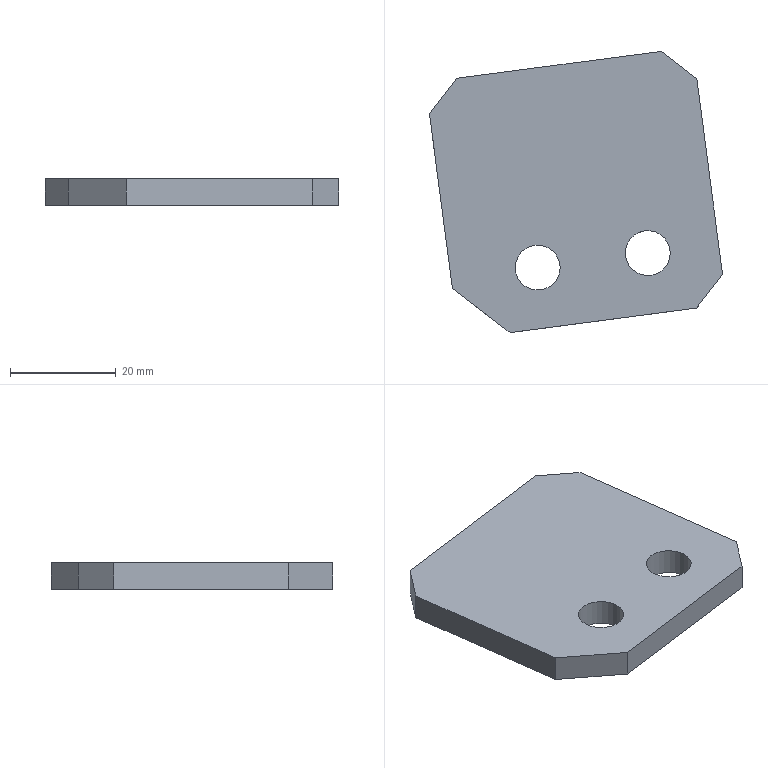Part | STEP file | gslz 2016.10.28-13_id538_x_t | 1 solid | 12 faces | box 55.431 x 53.187 x 5 mm | volume 11431 mm3 | plane 10 | cylinder 2 | commonest cylinder face diameters 8.5 x2
STEP:
#1=CARTESIAN_POINT('',(0.,0.,0.));
#2=DIRECTION('',(0.,0.,1.));
#3=DIRECTION('',(1.,0.,0.));
#4=AXIS2_PLACEMENT_3D('',#1,#2,#3);
#5=CARTESIAN_POINT('',(79.888,120.388,-99.));
#6=VERTEX_POINT('',#5);
#7=CARTESIAN_POINT('',(41.221,115.298,-99.));
#8=VERTEX_POINT('',#7);
#9=CARTESIAN_POINT('',(-1381.417,-71.996,-99.));
#10=DIRECTION('',(-0.9914,-0.1305,0.));
#11=VECTOR('',#10,1.);
#12=LINE('',#9,#11);
#13=CARTESIAN_POINT('',(-1381.417,-71.996,-99.));
#14=DIRECTION('',(-0.1305,0.9914,0.));
#15=DIRECTION('',(-0.9914,-0.1305,0.));
#16=AXIS2_PLACEMENT_3D('',#13,#14,#15);
#17=PLANE('',#16);
#18=CARTESIAN_POINT('',(0.,0.));
#19=DIRECTION('',(1.,0.));
#20=VECTOR('',#19,1.);
#21=LINE('',#18,#20);
#22=(GEOMETRIC_REPRESENTATION_CONTEXT(2)PARAMETRIC_REPRESENTATION_CONTEXT()REPRESENTATION_CONTEXT('',''));
#23=DEFINITIONAL_REPRESENTATION('',(#21),#22);
#24=PCURVE('',#17,#23);
#25=CARTESIAN_POINT('',(-1376.131,-112.149,-99.));
#26=DIRECTION('',(0.,0.,-1.));
#27=DIRECTION('',(-1.,0.,0.));
#28=AXIS2_PLACEMENT_3D('',#25,#26,#27);
#29=PLANE('',#28);
#30=CARTESIAN_POINT('',(5.286,40.154));
#31=DIRECTION('',(0.9914,-0.1305));
#32=VECTOR('',#31,1.);
#33=LINE('',#30,#32);
#34=(GEOMETRIC_REPRESENTATION_CONTEXT(2)PARAMETRIC_REPRESENTATION_CONTEXT()REPRESENTATION_CONTEXT('',''));
#35=DEFINITIONAL_REPRESENTATION('',(#33),#34);
#36=PCURVE('',#29,#35);
#37=SURFACE_CURVE('',#12,(#24,#36),.PCURVE_S1.);
#38=EDGE_CURVE('',#6,#8,#37,.T.);
#39=ORIENTED_EDGE('',*,*,#38,.T.);
#40=CARTESIAN_POINT('',(41.221,115.298,-94.));
#41=VERTEX_POINT('',#40);
#42=CARTESIAN_POINT('',(41.221,115.298,-94.));
#43=DIRECTION('',(0.,0.,1.));
#44=VECTOR('',#43,1.);
#45=LINE('',#42,#44);
#46=CARTESIAN_POINT('',(-1434.914,5.));
#47=DIRECTION('',(0.,1.));
#48=VECTOR('',#47,1.);
#49=LINE('',#46,#48);
#50=(GEOMETRIC_REPRESENTATION_CONTEXT(2)PARAMETRIC_REPRESENTATION_CONTEXT()REPRESENTATION_CONTEXT('',''));
#51=DEFINITIONAL_REPRESENTATION('',(#49),#50);
#52=PCURVE('',#17,#51);
#53=CARTESIAN_POINT('',(36.056,108.566,-267.));
#54=DIRECTION('',(0.7934,-0.6088,0.));
#55=DIRECTION('',(0.,0.,-1.));
#56=AXIS2_PLACEMENT_3D('',#53,#54,#55);
#57=PLANE('',#56);
#58=CARTESIAN_POINT('',(-173.,8.485));
#59=DIRECTION('',(-1.,0.));
#60=VECTOR('',#59,1.);
#61=LINE('',#58,#60);
#62=(GEOMETRIC_REPRESENTATION_CONTEXT(2)PARAMETRIC_REPRESENTATION_CONTEXT()REPRESENTATION_CONTEXT('',''));
#63=DEFINITIONAL_REPRESENTATION('',(#61),#62);
#64=PCURVE('',#57,#63);
#65=SURFACE_CURVE('',#45,(#52,#64),.PCURVE_S1.);
#66=EDGE_CURVE('',#8,#41,#65,.T.);
#67=ORIENTED_EDGE('',*,*,#66,.T.);
#68=CARTESIAN_POINT('',(79.888,120.388,-94.));
#69=VERTEX_POINT('',#68);
#70=CARTESIAN_POINT('',(-1381.417,-71.996,-94.));
#71=DIRECTION('',(-0.9914,-0.1305,0.));
#72=VECTOR('',#71,1.);
#73=LINE('',#70,#72);
#74=CARTESIAN_POINT('',(0.,5.));
#75=DIRECTION('',(1.,0.));
#76=VECTOR('',#75,1.);
#77=LINE('',#74,#76);
#78=(GEOMETRIC_REPRESENTATION_CONTEXT(2)PARAMETRIC_REPRESENTATION_CONTEXT()REPRESENTATION_CONTEXT('',''));
#79=DEFINITIONAL_REPRESENTATION('',(#77),#78);
#80=PCURVE('',#17,#79);
#81=CARTESIAN_POINT('',(-1376.131,-112.149,-94.));
#82=DIRECTION('',(0.,0.,-1.));
#83=DIRECTION('',(-1.,0.,0.));
#84=AXIS2_PLACEMENT_3D('',#81,#82,#83);
#85=PLANE('',#84);
#86=CARTESIAN_POINT('',(5.286,40.154));
#87=DIRECTION('',(0.9914,-0.1305));
#88=VECTOR('',#87,1.);
#89=LINE('',#86,#88);
#90=(GEOMETRIC_REPRESENTATION_CONTEXT(2)PARAMETRIC_REPRESENTATION_CONTEXT()REPRESENTATION_CONTEXT('',''));
#91=DEFINITIONAL_REPRESENTATION('',(#89),#90);
#92=PCURVE('',#85,#91);
#93=SURFACE_CURVE('',#73,(#80,#92),.PCURVE_S1.);
#94=EDGE_CURVE('',#69,#41,#93,.T.);
#95=ORIENTED_EDGE('',*,*,#94,.F.);
#96=CARTESIAN_POINT('',(79.888,120.388,-99.));
#97=DIRECTION('',(0.,0.,-1.));
#98=VECTOR('',#97,1.);
#99=LINE('',#96,#98);
#100=CARTESIAN_POINT('',(-1473.914,0.));
#101=DIRECTION('',(0.,-1.));
#102=VECTOR('',#101,1.);
#103=LINE('',#100,#102);
#104=(GEOMETRIC_REPRESENTATION_CONTEXT(2)PARAMETRIC_REPRESENTATION_CONTEXT()REPRESENTATION_CONTEXT('',''));
#105=DEFINITIONAL_REPRESENTATION('',(#103),#104);
#106=PCURVE('',#17,#105);
#107=CARTESIAN_POINT('',(86.619,115.223,-267.));
#108=DIRECTION('',(0.6088,0.7934,0.));
#109=DIRECTION('',(0.,0.,-1.));
#110=AXIS2_PLACEMENT_3D('',#107,#108,#109);
#111=PLANE('',#110);
#112=CARTESIAN_POINT('',(-168.,8.485));
#113=DIRECTION('',(1.,0.));
#114=VECTOR('',#113,1.);
#115=LINE('',#112,#114);
#116=(GEOMETRIC_REPRESENTATION_CONTEXT(2)PARAMETRIC_REPRESENTATION_CONTEXT()REPRESENTATION_CONTEXT('',''));
#117=DEFINITIONAL_REPRESENTATION('',(#115),#116);
#118=PCURVE('',#111,#117);
#119=SURFACE_CURVE('',#99,(#106,#118),.PCURVE_S1.);
#120=EDGE_CURVE('',#69,#6,#119,.T.);
#121=ORIENTED_EDGE('',*,*,#120,.T.);
#122=EDGE_LOOP('',(#39,#67,#95,#121));
#123=FACE_BOUND('',#122,.T.);
#124=ADVANCED_FACE('',(#123),#17,.T.);
#125=CARTESIAN_POINT('',(91.487,78.249,-99.));
#126=VERTEX_POINT('',#125);
#127=CARTESIAN_POINT('',(86.619,115.223,-99.));
#128=VERTEX_POINT('',#127);
#129=CARTESIAN_POINT('',(91.123,81.018,-99.));
#130=DIRECTION('',(-0.1305,0.9914,0.));
#131=VECTOR('',#130,1.);
#132=LINE('',#129,#131);
#133=CARTESIAN_POINT('',(91.123,81.018,-267.));
#134=DIRECTION('',(-0.9914,-0.1305,0.));
#135=DIRECTION('',(0.1305,-0.9914,0.));
#136=AXIS2_PLACEMENT_3D('',#133,#134,#135);
#137=PLANE('',#136);
#138=CARTESIAN_POINT('',(0.,168.));
#139=DIRECTION('',(-1.,0.));
#140=VECTOR('',#139,1.);
#141=LINE('',#138,#140);
#142=(GEOMETRIC_REPRESENTATION_CONTEXT(2)PARAMETRIC_REPRESENTATION_CONTEXT()REPRESENTATION_CONTEXT('',''));
#143=DEFINITIONAL_REPRESENTATION('',(#141),#142);
#144=PCURVE('',#137,#143);
#145=CARTESIAN_POINT('',(-1467.254,193.167));
#146=DIRECTION('',(0.1305,0.9914));
#147=VECTOR('',#146,1.);
#148=LINE('',#145,#147);
#149=(GEOMETRIC_REPRESENTATION_CONTEXT(2)PARAMETRIC_REPRESENTATION_CONTEXT()REPRESENTATION_CONTEXT('',''));
#150=DEFINITIONAL_REPRESENTATION('',(#148),#149);
#151=PCURVE('',#29,#150);
#152=SURFACE_CURVE('',#132,(#144,#151),.PCURVE_S1.);
#153=EDGE_CURVE('',#126,#128,#152,.T.);
#154=ORIENTED_EDGE('',*,*,#153,.T.);
#155=CARTESIAN_POINT('',(86.619,115.223,-94.));
#156=VERTEX_POINT('',#155);
#157=CARTESIAN_POINT('',(86.619,115.223,-267.));
#158=DIRECTION('',(0.,0.,1.));
#159=VECTOR('',#158,1.);
#160=LINE('',#157,#159);
#161=CARTESIAN_POINT('',(-34.5,0.));
#162=DIRECTION('',(0.,1.));
#163=VECTOR('',#162,1.);
#164=LINE('',#161,#163);
#165=(GEOMETRIC_REPRESENTATION_CONTEXT(2)PARAMETRIC_REPRESENTATION_CONTEXT()REPRESENTATION_CONTEXT('',''));
#166=DEFINITIONAL_REPRESENTATION('',(#164),#165);
#167=PCURVE('',#137,#166);
#168=CARTESIAN_POINT('',(0.,0.));
#169=DIRECTION('',(-1.,0.));
#170=VECTOR('',#169,1.);
#171=LINE('',#168,#170);
#172=(GEOMETRIC_REPRESENTATION_CONTEXT(2)PARAMETRIC_REPRESENTATION_CONTEXT()REPRESENTATION_CONTEXT('',''));
#173=DEFINITIONAL_REPRESENTATION('',(#171),#172);
#174=PCURVE('',#111,#173);
#175=SURFACE_CURVE('',#160,(#167,#174),.PCURVE_S1.);
#176=EDGE_CURVE('',#128,#156,#175,.T.);
#177=ORIENTED_EDGE('',*,*,#176,.T.);
#178=CARTESIAN_POINT('',(91.487,78.249,-94.));
#179=VERTEX_POINT('',#178);
#180=CARTESIAN_POINT('',(91.123,81.018,-94.));
#181=DIRECTION('',(-0.1305,0.9914,0.));
#182=VECTOR('',#181,1.);
#183=LINE('',#180,#182);
#184=CARTESIAN_POINT('',(0.,173.));
#185=DIRECTION('',(-1.,0.));
#186=VECTOR('',#185,1.);
#187=LINE('',#184,#186);
#188=(GEOMETRIC_REPRESENTATION_CONTEXT(2)PARAMETRIC_REPRESENTATION_CONTEXT()REPRESENTATION_CONTEXT('',''));
#189=DEFINITIONAL_REPRESENTATION('',(#187),#188);
#190=PCURVE('',#137,#189);
#191=CARTESIAN_POINT('',(-1467.254,193.167));
#192=DIRECTION('',(0.1305,0.9914));
#193=VECTOR('',#192,1.);
#194=LINE('',#191,#193);
#195=(GEOMETRIC_REPRESENTATION_CONTEXT(2)PARAMETRIC_REPRESENTATION_CONTEXT()REPRESENTATION_CONTEXT('',''));
#196=DEFINITIONAL_REPRESENTATION('',(#194),#195);
#197=PCURVE('',#85,#196);
#198=SURFACE_CURVE('',#183,(#190,#197),.PCURVE_S1.);
#199=EDGE_CURVE('',#179,#156,#198,.T.);
#200=ORIENTED_EDGE('',*,*,#199,.F.);
#201=CARTESIAN_POINT('',(91.487,78.249,-267.));
#202=DIRECTION('',(0.,0.,-1.));
#203=VECTOR('',#202,1.);
#204=LINE('',#201,#203);
#205=CARTESIAN_POINT('',(2.793,0.));
#206=DIRECTION('',(0.,-1.));
#207=VECTOR('',#206,1.);
#208=LINE('',#205,#207);
#209=(GEOMETRIC_REPRESENTATION_CONTEXT(2)PARAMETRIC_REPRESENTATION_CONTEXT()REPRESENTATION_CONTEXT('',''));
#210=DEFINITIONAL_REPRESENTATION('',(#208),#209);
#211=PCURVE('',#137,#210);
#212=CARTESIAN_POINT('',(91.613,78.413,-267.));
#213=DIRECTION('',(-0.7934,0.6088,0.));
#214=DIRECTION('',(0.,0.,-1.));
#215=AXIS2_PLACEMENT_3D('',#212,#213,#214);
#216=PLANE('',#215);
#217=CARTESIAN_POINT('',(0.,0.2071));
#218=DIRECTION('',(1.,0.));
#219=VECTOR('',#218,1.);
#220=LINE('',#217,#219);
#221=(GEOMETRIC_REPRESENTATION_CONTEXT(2)PARAMETRIC_REPRESENTATION_CONTEXT()REPRESENTATION_CONTEXT('',''));
#222=DEFINITIONAL_REPRESENTATION('',(#220),#221);
#223=PCURVE('',#216,#222);
#224=SURFACE_CURVE('',#204,(#211,#223),.PCURVE_S1.);
#225=EDGE_CURVE('',#179,#126,#224,.T.);
#226=ORIENTED_EDGE('',*,*,#225,.T.);
#227=EDGE_LOOP('',(#154,#177,#200,#226));
#228=FACE_BOUND('',#227,.T.);
#229=ADVANCED_FACE('',(#228),#137,.F.);
#230=CARTESIAN_POINT('',(86.574,71.846,-94.));
#231=VERTEX_POINT('',#230);
#232=CARTESIAN_POINT('',(51.292,67.201,-94.));
#233=VERTEX_POINT('',#232);
#234=CARTESIAN_POINT('',(-1375.022,-120.577,-94.));
#235=DIRECTION('',(-0.9914,-0.1305,0.));
#236=VECTOR('',#235,1.);
#237=LINE('',#234,#236);
#238=CARTESIAN_POINT('',(-1375.022,-120.577,-267.));
#239=DIRECTION('',(-0.1305,0.9914,0.));
#240=DIRECTION('',(-0.9914,-0.1305,0.));
#241=AXIS2_PLACEMENT_3D('',#238,#239,#240);
#242=PLANE('',#241);
#243=CARTESIAN_POINT('',(0.,173.));
#244=DIRECTION('',(1.,0.));
#245=VECTOR('',#244,1.);
#246=LINE('',#243,#245);
#247=(GEOMETRIC_REPRESENTATION_CONTEXT(2)PARAMETRIC_REPRESENTATION_CONTEXT()REPRESENTATION_CONTEXT('',''));
#248=DEFINITIONAL_REPRESENTATION('',(#246),#247);
#249=PCURVE('',#242,#248);
#250=CARTESIAN_POINT('',(-1.109,-8.427));
#251=DIRECTION('',(0.9914,-0.1305));
#252=VECTOR('',#251,1.);
#253=LINE('',#250,#252);
#254=(GEOMETRIC_REPRESENTATION_CONTEXT(2)PARAMETRIC_REPRESENTATION_CONTEXT()REPRESENTATION_CONTEXT('',''));
#255=DEFINITIONAL_REPRESENTATION('',(#253),#254);
#256=PCURVE('',#85,#255);
#257=SURFACE_CURVE('',#237,(#249,#256),.PCURVE_S1.);
#258=EDGE_CURVE('',#231,#233,#257,.T.);
#259=ORIENTED_EDGE('',*,*,#258,.T.);
#260=CARTESIAN_POINT('',(51.292,67.201,-99.));
#261=VERTEX_POINT('',#260);
#262=CARTESIAN_POINT('',(51.292,67.201,-267.));
#263=DIRECTION('',(0.,0.,-1.));
#264=VECTOR('',#263,1.);
#265=LINE('',#262,#264);
#266=CARTESIAN_POINT('',(-1438.622,0.));
#267=DIRECTION('',(0.,-1.));
#268=VECTOR('',#267,1.);
#269=LINE('',#266,#268);
#270=(GEOMETRIC_REPRESENTATION_CONTEXT(2)PARAMETRIC_REPRESENTATION_CONTEXT()REPRESENTATION_CONTEXT('',''));
#271=DEFINITIONAL_REPRESENTATION('',(#269),#270);
#272=PCURVE('',#242,#271);
#273=CARTESIAN_POINT('',(40.237,75.684,-267.));
#274=DIRECTION('',(-0.6088,-0.7934,0.));
#275=DIRECTION('',(0.,0.,-1.));
#276=AXIS2_PLACEMENT_3D('',#273,#274,#275);
#277=PLANE('',#276);
#278=CARTESIAN_POINT('',(0.,13.935));
#279=DIRECTION('',(1.,0.));
#280=VECTOR('',#279,1.);
#281=LINE('',#278,#280);
#282=(GEOMETRIC_REPRESENTATION_CONTEXT(2)PARAMETRIC_REPRESENTATION_CONTEXT()REPRESENTATION_CONTEXT('',''));
#283=DEFINITIONAL_REPRESENTATION('',(#281),#282);
#284=PCURVE('',#277,#283);
#285=SURFACE_CURVE('',#265,(#272,#284),.PCURVE_S1.);
#286=EDGE_CURVE('',#233,#261,#285,.T.);
#287=ORIENTED_EDGE('',*,*,#286,.T.);
#288=CARTESIAN_POINT('',(86.574,71.846,-99.));
#289=VERTEX_POINT('',#288);
#290=CARTESIAN_POINT('',(-1375.022,-120.577,-99.));
#291=DIRECTION('',(-0.9914,-0.1305,0.));
#292=VECTOR('',#291,1.);
#293=LINE('',#290,#292);
#294=CARTESIAN_POINT('',(0.,168.));
#295=DIRECTION('',(1.,0.));
#296=VECTOR('',#295,1.);
#297=LINE('',#294,#296);
#298=(GEOMETRIC_REPRESENTATION_CONTEXT(2)PARAMETRIC_REPRESENTATION_CONTEXT()REPRESENTATION_CONTEXT('',''));
#299=DEFINITIONAL_REPRESENTATION('',(#297),#298);
#300=PCURVE('',#242,#299);
#301=CARTESIAN_POINT('',(-1.109,-8.427));
#302=DIRECTION('',(0.9914,-0.1305));
#303=VECTOR('',#302,1.);
#304=LINE('',#301,#303);
#305=(GEOMETRIC_REPRESENTATION_CONTEXT(2)PARAMETRIC_REPRESENTATION_CONTEXT()REPRESENTATION_CONTEXT('',''));
#306=DEFINITIONAL_REPRESENTATION('',(#304),#305);
#307=PCURVE('',#29,#306);
#308=SURFACE_CURVE('',#293,(#300,#307),.PCURVE_S1.);
#309=EDGE_CURVE('',#289,#261,#308,.T.);
#310=ORIENTED_EDGE('',*,*,#309,.F.);
#311=CARTESIAN_POINT('',(86.574,71.846,-267.));
#312=DIRECTION('',(0.,0.,1.));
#313=VECTOR('',#312,1.);
#314=LINE('',#311,#313);
#315=CARTESIAN_POINT('',(-1474.207,0.));
#316=DIRECTION('',(0.,1.));
#317=VECTOR('',#316,1.);
#318=LINE('',#315,#317);
#319=(GEOMETRIC_REPRESENTATION_CONTEXT(2)PARAMETRIC_REPRESENTATION_CONTEXT()REPRESENTATION_CONTEXT('',''));
#320=DEFINITIONAL_REPRESENTATION('',(#318),#319);
#321=PCURVE('',#242,#320);
#322=CARTESIAN_POINT('',(0.,8.278));
#323=DIRECTION('',(-1.,0.));
#324=VECTOR('',#323,1.);
#325=LINE('',#322,#324);
#326=(GEOMETRIC_REPRESENTATION_CONTEXT(2)PARAMETRIC_REPRESENTATION_CONTEXT()REPRESENTATION_CONTEXT('',''));
#327=DEFINITIONAL_REPRESENTATION('',(#325),#326);
#328=PCURVE('',#216,#327);
#329=SURFACE_CURVE('',#314,(#321,#328),.PCURVE_S1.);
#330=EDGE_CURVE('',#289,#231,#329,.T.);
#331=ORIENTED_EDGE('',*,*,#330,.T.);
#332=EDGE_LOOP('',(#259,#287,#310,#331));
#333=FACE_BOUND('',#332,.T.);
#334=ADVANCED_FACE('',(#333),#242,.F.);
#335=CARTESIAN_POINT('',(40.401,75.558,-94.));
#336=VERTEX_POINT('',#335);
#337=CARTESIAN_POINT('',(36.056,108.566,-94.));
#338=VERTEX_POINT('',#337);
#339=CARTESIAN_POINT('',(40.559,74.361,-94.));
#340=DIRECTION('',(-0.1305,0.9914,0.));
#341=VECTOR('',#340,1.);
#342=LINE('',#339,#341);
#343=CARTESIAN_POINT('',(40.559,74.361,-267.));
#344=DIRECTION('',(-0.9914,-0.1305,0.));
#345=DIRECTION('',(0.1305,-0.9914,0.));
#346=AXIS2_PLACEMENT_3D('',#343,#344,#345);
#347=PLANE('',#346);
#348=CARTESIAN_POINT('',(0.,173.));
#349=DIRECTION('',(-1.,0.));
#350=VECTOR('',#349,1.);
#351=LINE('',#348,#350);
#352=(GEOMETRIC_REPRESENTATION_CONTEXT(2)PARAMETRIC_REPRESENTATION_CONTEXT()REPRESENTATION_CONTEXT('',''));
#353=DEFINITIONAL_REPRESENTATION('',(#351),#352);
#354=PCURVE('',#347,#353);
#355=CARTESIAN_POINT('',(-1416.69,186.51));
#356=DIRECTION('',(0.1305,0.9914));
#357=VECTOR('',#356,1.);
#358=LINE('',#355,#357);
#359=(GEOMETRIC_REPRESENTATION_CONTEXT(2)PARAMETRIC_REPRESENTATION_CONTEXT()REPRESENTATION_CONTEXT('',''));
#360=DEFINITIONAL_REPRESENTATION('',(#358),#359);
#361=PCURVE('',#85,#360);
#362=SURFACE_CURVE('',#342,(#354,#361),.PCURVE_S1.);
#363=EDGE_CURVE('',#336,#338,#362,.T.);
#364=ORIENTED_EDGE('',*,*,#363,.T.);
#365=CARTESIAN_POINT('',(36.056,108.566,-99.));
#366=VERTEX_POINT('',#365);
#367=CARTESIAN_POINT('',(36.056,108.566,-99.));
#368=DIRECTION('',(0.,0.,-1.));
#369=VECTOR('',#368,1.);
#370=LINE('',#367,#369);
#371=CARTESIAN_POINT('',(-34.5,168.));
#372=DIRECTION('',(0.,-1.));
#373=VECTOR('',#372,1.);
#374=LINE('',#371,#373);
#375=(GEOMETRIC_REPRESENTATION_CONTEXT(2)PARAMETRIC_REPRESENTATION_CONTEXT()REPRESENTATION_CONTEXT('',''));
#376=DEFINITIONAL_REPRESENTATION('',(#374),#375);
#377=PCURVE('',#347,#376);
#378=CARTESIAN_POINT('',(-168.,0.));
#379=DIRECTION('',(1.,0.));
#380=VECTOR('',#379,1.);
#381=LINE('',#378,#380);
#382=(GEOMETRIC_REPRESENTATION_CONTEXT(2)PARAMETRIC_REPRESENTATION_CONTEXT()REPRESENTATION_CONTEXT('',''));
#383=DEFINITIONAL_REPRESENTATION('',(#381),#382);
#384=PCURVE('',#57,#383);
#385=SURFACE_CURVE('',#370,(#377,#384),.PCURVE_S1.);
#386=EDGE_CURVE('',#338,#366,#385,.T.);
#387=ORIENTED_EDGE('',*,*,#386,.T.);
#388=CARTESIAN_POINT('',(40.401,75.558,-99.));
#389=VERTEX_POINT('',#388);
#390=CARTESIAN_POINT('',(40.559,74.361,-99.));
#391=DIRECTION('',(-0.1305,0.9914,0.));
#392=VECTOR('',#391,1.);
#393=LINE('',#390,#392);
#394=CARTESIAN_POINT('',(0.,168.));
#395=DIRECTION('',(-1.,0.));
#396=VECTOR('',#395,1.);
#397=LINE('',#394,#396);
#398=(GEOMETRIC_REPRESENTATION_CONTEXT(2)PARAMETRIC_REPRESENTATION_CONTEXT()REPRESENTATION_CONTEXT('',''));
#399=DEFINITIONAL_REPRESENTATION('',(#397),#398);
#400=PCURVE('',#347,#399);
#401=CARTESIAN_POINT('',(-1416.69,186.51));
#402=DIRECTION('',(0.1305,0.9914));
#403=VECTOR('',#402,1.);
#404=LINE('',#401,#403);
#405=(GEOMETRIC_REPRESENTATION_CONTEXT(2)PARAMETRIC_REPRESENTATION_CONTEXT()REPRESENTATION_CONTEXT('',''));
#406=DEFINITIONAL_REPRESENTATION('',(#404),#405);
#407=PCURVE('',#29,#406);
#408=SURFACE_CURVE('',#393,(#400,#407),.PCURVE_S1.);
#409=EDGE_CURVE('',#389,#366,#408,.T.);
#410=ORIENTED_EDGE('',*,*,#409,.F.);
#411=CARTESIAN_POINT('',(40.401,75.558,-267.));
#412=DIRECTION('',(0.,0.,1.));
#413=VECTOR('',#412,1.);
#414=LINE('',#411,#413);
#415=CARTESIAN_POINT('',(-1.207,0.));
#416=DIRECTION('',(0.,1.));
#417=VECTOR('',#416,1.);
#418=LINE('',#415,#417);
#419=(GEOMETRIC_REPRESENTATION_CONTEXT(2)PARAMETRIC_REPRESENTATION_CONTEXT()REPRESENTATION_CONTEXT('',''));
#420=DEFINITIONAL_REPRESENTATION('',(#418),#419);
#421=PCURVE('',#347,#420);
#422=CARTESIAN_POINT('',(0.,0.2071));
#423=DIRECTION('',(-1.,0.));
#424=VECTOR('',#423,1.);
#425=LINE('',#422,#424);
#426=(GEOMETRIC_REPRESENTATION_CONTEXT(2)PARAMETRIC_REPRESENTATION_CONTEXT()REPRESENTATION_CONTEXT('',''));
#427=DEFINITIONAL_REPRESENTATION('',(#425),#426);
#428=PCURVE('',#277,#427);
#429=SURFACE_CURVE('',#414,(#421,#428),.PCURVE_S1.);
#430=EDGE_CURVE('',#389,#336,#429,.T.);
#431=ORIENTED_EDGE('',*,*,#430,.T.);
#432=EDGE_LOOP('',(#364,#387,#410,#431));
#433=FACE_BOUND('',#432,.T.);
#434=ADVANCED_FACE('',(#433),#347,.T.);
#435=CARTESIAN_POINT('',(52.276,79.489,-99.));
#436=VERTEX_POINT('',#435);
#437=CARTESIAN_POINT('',(56.526,79.489,-99.));
#438=DIRECTION('',(0.,0.,-1.));
#439=DIRECTION('',(-1.,0.,0.));
#440=AXIS2_PLACEMENT_3D('',#437,#438,#439);
#441=CIRCLE('',#440,4.25);
#442=CARTESIAN_POINT('',(56.526,79.489,-99.));
#443=DIRECTION('',(0.,0.,1.));
#444=DIRECTION('',(1.,0.,0.));
#445=AXIS2_PLACEMENT_3D('',#442,#443,#444);
#446=CYLINDRICAL_SURFACE('',#445,4.25);
#447=CARTESIAN_POINT('',(9.425,0.));
#448=DIRECTION('',(-1.,0.));
#449=VECTOR('',#448,1.);
#450=LINE('',#447,#449);
#451=(GEOMETRIC_REPRESENTATION_CONTEXT(2)PARAMETRIC_REPRESENTATION_CONTEXT()REPRESENTATION_CONTEXT('',''));
#452=DEFINITIONAL_REPRESENTATION('',(#450),#451);
#453=PCURVE('',#446,#452);
#454=CARTESIAN_POINT('',(-1432.657,191.638));
#455=DIRECTION('',(1.,0.));
#456=AXIS2_PLACEMENT_2D('',#454,#455);
#457=CIRCLE('',#456,4.25);
#458=(GEOMETRIC_REPRESENTATION_CONTEXT(2)PARAMETRIC_REPRESENTATION_CONTEXT()REPRESENTATION_CONTEXT('',''));
#459=DEFINITIONAL_REPRESENTATION('',(#457),#458);
#460=PCURVE('',#29,#459);
#461=SURFACE_CURVE('',#441,(#453,#460),.PCURVE_S1.);
#462=EDGE_CURVE('',#436,#436,#461,.T.);
#463=ORIENTED_EDGE('',*,*,#462,.F.);
#464=CARTESIAN_POINT('',(52.276,79.489,-94.));
#465=VERTEX_POINT('',#464);
#466=CARTESIAN_POINT('',(52.276,79.489,-99.));
#467=CARTESIAN_POINT('',(52.276,79.489,-94.));
#468=B_SPLINE_CURVE_WITH_KNOTS('',1,(#466,#467),.UNSPECIFIED.,.F.,.F.,(2,2),(0.,5.),.PIECEWISE_BEZIER_KNOTS.);
#469=CARTESIAN_POINT('',(9.425,0.));
#470=DIRECTION('',(0.,1.));
#471=VECTOR('',#470,1.);
#472=LINE('',#469,#471);
#473=(GEOMETRIC_REPRESENTATION_CONTEXT(2)PARAMETRIC_REPRESENTATION_CONTEXT()REPRESENTATION_CONTEXT('',''));
#474=DEFINITIONAL_REPRESENTATION('',(#472),#473);
#475=PCURVE('',#446,#474);
#476=CARTESIAN_POINT('',(3.142,0.));
#477=DIRECTION('',(0.,1.));
#478=VECTOR('',#477,1.);
#479=LINE('',#476,#478);
#480=(GEOMETRIC_REPRESENTATION_CONTEXT(2)PARAMETRIC_REPRESENTATION_CONTEXT()REPRESENTATION_CONTEXT('',''));
#481=DEFINITIONAL_REPRESENTATION('',(#479),#480);
#482=PCURVE('',#446,#481);
#483=SEAM_CURVE('',#468,(#475,#482),.PCURVE_S1.);
#484=EDGE_CURVE('',#436,#465,#483,.T.);
#485=ORIENTED_EDGE('',*,*,#484,.T.);
#486=CARTESIAN_POINT('',(56.526,79.489,-94.));
#487=DIRECTION('',(0.,0.,-1.));
#488=DIRECTION('',(-1.,0.,0.));
#489=AXIS2_PLACEMENT_3D('',#486,#487,#488);
#490=CIRCLE('',#489,4.25);
#491=CARTESIAN_POINT('',(9.425,5.));
#492=DIRECTION('',(-1.,0.));
#493=VECTOR('',#492,1.);
#494=LINE('',#491,#493);
#495=(GEOMETRIC_REPRESENTATION_CONTEXT(2)PARAMETRIC_REPRESENTATION_CONTEXT()REPRESENTATION_CONTEXT('',''));
#496=DEFINITIONAL_REPRESENTATION('',(#494),#495);
#497=PCURVE('',#446,#496);
#498=CARTESIAN_POINT('',(-1432.657,191.638));
#499=DIRECTION('',(1.,0.));
#500=AXIS2_PLACEMENT_2D('',#498,#499);
#501=CIRCLE('',#500,4.25);
#502=(GEOMETRIC_REPRESENTATION_CONTEXT(2)PARAMETRIC_REPRESENTATION_CONTEXT()REPRESENTATION_CONTEXT('',''));
#503=DEFINITIONAL_REPRESENTATION('',(#501),#502);
#504=PCURVE('',#85,#503);
#505=SURFACE_CURVE('',#490,(#497,#504),.PCURVE_S1.);
#506=EDGE_CURVE('',#465,#465,#505,.T.);
#507=ORIENTED_EDGE('',*,*,#506,.T.);
#508=ORIENTED_EDGE('',*,*,#484,.F.);
#509=EDGE_LOOP('',(#463,#485,#507,#508));
#510=FACE_BOUND('',#509,.F.);
#511=ADVANCED_FACE('',(#510),#446,.F.);
#512=CARTESIAN_POINT('',(81.452,83.33,-99.));
#513=VERTEX_POINT('',#512);
#514=CARTESIAN_POINT('',(77.346,82.23,-99.));
#515=DIRECTION('',(0.,0.,1.));
#516=DIRECTION('',(0.9659,0.2588,0.));
#517=AXIS2_PLACEMENT_3D('',#514,#515,#516);
#518=CIRCLE('',#517,4.25);
#519=CARTESIAN_POINT('',(77.346,82.23,-99.));
#520=DIRECTION('',(0.,0.,1.));
#521=DIRECTION('',(1.,0.,0.));
#522=AXIS2_PLACEMENT_3D('',#519,#520,#521);
#523=CYLINDRICAL_SURFACE('',#522,4.25);
#524=CARTESIAN_POINT('',(0.2618,0.));
#525=DIRECTION('',(1.,0.));
#526=VECTOR('',#525,1.);
#527=LINE('',#524,#526);
#528=(GEOMETRIC_REPRESENTATION_CONTEXT(2)PARAMETRIC_REPRESENTATION_CONTEXT()REPRESENTATION_CONTEXT('',''));
#529=DEFINITIONAL_REPRESENTATION('',(#527),#528);
#530=PCURVE('',#523,#529);
#531=CARTESIAN_POINT('',(-1457.583,195.48));
#532=CARTESIAN_POINT('',(-1455.678,202.59));
#533=CARTESIAN_POINT('',(-1450.472,197.385));
#534=CARTESIAN_POINT('',(-1445.267,192.18));
#535=CARTESIAN_POINT('',(-1452.378,190.274));
#536=CARTESIAN_POINT('',(-1459.488,188.369));
#537=CARTESIAN_POINT('',(-1457.583,195.48));
#538=(BOUNDED_CURVE()B_SPLINE_CURVE(2,(#531,#532,#533,#534,#535,#536,#537),.UNSPECIFIED.,.T.,.F.)B_SPLINE_CURVE_WITH_KNOTS((1,2,2,2,2,1),(-2.094,0.,2.094,4.189,6.283,8.378),.UNSPECIFIED.)CURVE()GEOMETRIC_REPRESENTATION_ITEM()RATIONAL_B_SPLINE_CURVE((1.,0.5,1.,0.5,1.,0.5,1.))REPRESENTATION_ITEM(''));
#539=(GEOMETRIC_REPRESENTATION_CONTEXT(2)PARAMETRIC_REPRESENTATION_CONTEXT()REPRESENTATION_CONTEXT('',''));
#540=DEFINITIONAL_REPRESENTATION('',(#538),#539);
#541=PCURVE('',#29,#540);
#542=SURFACE_CURVE('',#518,(#530,#541),.PCURVE_S1.);
#543=EDGE_CURVE('',#513,#513,#542,.T.);
#544=ORIENTED_EDGE('',*,*,#543,.T.);
#545=CARTESIAN_POINT('',(81.452,83.33,-94.));
#546=VERTEX_POINT('',#545);
#547=CARTESIAN_POINT('',(81.452,83.33,-99.));
#548=CARTESIAN_POINT('',(81.452,83.33,-94.));
#549=B_SPLINE_CURVE_WITH_KNOTS('',1,(#547,#548),.UNSPECIFIED.,.F.,.F.,(2,2),(0.,5.),.PIECEWISE_BEZIER_KNOTS.);
#550=CARTESIAN_POINT('',(6.545,0.));
#551=DIRECTION('',(0.,1.));
#552=VECTOR('',#551,1.);
#553=LINE('',#550,#552);
#554=(GEOMETRIC_REPRESENTATION_CONTEXT(2)PARAMETRIC_REPRESENTATION_CONTEXT()REPRESENTATION_CONTEXT('',''));
#555=DEFINITIONAL_REPRESENTATION('',(#553),#554);
#556=PCURVE('',#523,#555);
#557=CARTESIAN_POINT('',(0.2618,0.));
#558=DIRECTION('',(0.,1.));
#559=VECTOR('',#558,1.);
#560=LINE('',#557,#559);
#561=(GEOMETRIC_REPRESENTATION_CONTEXT(2)PARAMETRIC_REPRESENTATION_CONTEXT()REPRESENTATION_CONTEXT('',''));
#562=DEFINITIONAL_REPRESENTATION('',(#560),#561);
#563=PCURVE('',#523,#562);
#564=SEAM_CURVE('',#549,(#556,#563),.PCURVE_S1.);
#565=EDGE_CURVE('',#513,#546,#564,.T.);
#566=ORIENTED_EDGE('',*,*,#565,.T.);
#567=CARTESIAN_POINT('',(77.346,82.23,-94.));
#568=DIRECTION('',(0.,0.,1.));
#569=DIRECTION('',(0.9659,0.2588,0.));
#570=AXIS2_PLACEMENT_3D('',#567,#568,#569);
#571=CIRCLE('',#570,4.25);
#572=CARTESIAN_POINT('',(0.2618,5.));
#573=DIRECTION('',(1.,0.));
#574=VECTOR('',#573,1.);
#575=LINE('',#572,#574);
#576=(GEOMETRIC_REPRESENTATION_CONTEXT(2)PARAMETRIC_REPRESENTATION_CONTEXT()REPRESENTATION_CONTEXT('',''));
#577=DEFINITIONAL_REPRESENTATION('',(#575),#576);
#578=PCURVE('',#523,#577);
#579=CARTESIAN_POINT('',(-1457.583,195.48));
#580=CARTESIAN_POINT('',(-1455.678,202.59));
#581=CARTESIAN_POINT('',(-1450.472,197.385));
#582=CARTESIAN_POINT('',(-1445.267,192.18));
#583=CARTESIAN_POINT('',(-1452.378,190.274));
#584=CARTESIAN_POINT('',(-1459.488,188.369));
#585=CARTESIAN_POINT('',(-1457.583,195.48));
#586=(BOUNDED_CURVE()B_SPLINE_CURVE(2,(#579,#580,#581,#582,#583,#584,#585),.UNSPECIFIED.,.T.,.F.)B_SPLINE_CURVE_WITH_KNOTS((1,2,2,2,2,1),(-2.094,0.,2.094,4.189,6.283,8.378),.UNSPECIFIED.)CURVE()GEOMETRIC_REPRESENTATION_ITEM()RATIONAL_B_SPLINE_CURVE((1.,0.5,1.,0.5,1.,0.5,1.))REPRESENTATION_ITEM(''));
#587=(GEOMETRIC_REPRESENTATION_CONTEXT(2)PARAMETRIC_REPRESENTATION_CONTEXT()REPRESENTATION_CONTEXT('',''));
#588=DEFINITIONAL_REPRESENTATION('',(#586),#587);
#589=PCURVE('',#85,#588);
#590=SURFACE_CURVE('',#571,(#578,#589),.PCURVE_S1.);
#591=EDGE_CURVE('',#546,#546,#590,.T.);
#592=ORIENTED_EDGE('',*,*,#591,.F.);
#593=ORIENTED_EDGE('',*,*,#565,.F.);
#594=EDGE_LOOP('',(#544,#566,#592,#593));
#595=FACE_BOUND('',#594,.F.);
#596=ADVANCED_FACE('',(#595),#523,.F.);
#597=ORIENTED_EDGE('',*,*,#409,.T.);
#598=CARTESIAN_POINT('',(-593.885,-712.388,-99.));
#599=DIRECTION('',(0.6088,0.7934,0.));
#600=VECTOR('',#599,1.);
#601=LINE('',#598,#600);
#602=CARTESIAN_POINT('',(-782.246,-600.239));
#603=DIRECTION('',(-0.6088,0.7934));
#604=VECTOR('',#603,1.);
#605=LINE('',#602,#604);
#606=(GEOMETRIC_REPRESENTATION_CONTEXT(2)PARAMETRIC_REPRESENTATION_CONTEXT()REPRESENTATION_CONTEXT('',''));
#607=DEFINITIONAL_REPRESENTATION('',(#605),#606);
#608=PCURVE('',#29,#607);
#609=CARTESIAN_POINT('',(-168.,-1034.79));
#610=DIRECTION('',(0.,1.));
#611=VECTOR('',#610,1.);
#612=LINE('',#609,#611);
#613=(GEOMETRIC_REPRESENTATION_CONTEXT(2)PARAMETRIC_REPRESENTATION_CONTEXT()REPRESENTATION_CONTEXT('',''));
#614=DEFINITIONAL_REPRESENTATION('',(#612),#613);
#615=PCURVE('',#57,#614);
#616=SURFACE_CURVE('',#601,(#608,#615),.PCURVE_S1.);
#617=EDGE_CURVE('',#366,#8,#616,.T.);
#618=ORIENTED_EDGE('',*,*,#617,.T.);
#619=ORIENTED_EDGE('',*,*,#38,.F.);
#620=CARTESIAN_POINT('',(-724.237,737.415,-99.));
#621=DIRECTION('',(0.7934,-0.6088,0.));
#622=VECTOR('',#621,1.);
#623=LINE('',#620,#622);
#624=CARTESIAN_POINT('',(-651.894,849.564));
#625=DIRECTION('',(-0.7934,-0.6088));
#626=VECTOR('',#625,1.);
#627=LINE('',#624,#626);
#628=(GEOMETRIC_REPRESENTATION_CONTEXT(2)PARAMETRIC_REPRESENTATION_CONTEXT()REPRESENTATION_CONTEXT('',''));
#629=DEFINITIONAL_REPRESENTATION('',(#627),#628);
#630=PCURVE('',#29,#629);
#631=CARTESIAN_POINT('',(-168.,1022.062));
#632=DIRECTION('',(0.,-1.));
#633=VECTOR('',#632,1.);
#634=LINE('',#631,#633);
#635=(GEOMETRIC_REPRESENTATION_CONTEXT(2)PARAMETRIC_REPRESENTATION_CONTEXT()REPRESENTATION_CONTEXT('',''));
#636=DEFINITIONAL_REPRESENTATION('',(#634),#635);
#637=PCURVE('',#111,#636);
#638=SURFACE_CURVE('',#623,(#630,#637),.PCURVE_S1.);
#639=EDGE_CURVE('',#6,#128,#638,.T.);
#640=ORIENTED_EDGE('',*,*,#639,.T.);
#641=ORIENTED_EDGE('',*,*,#153,.F.);
#642=CARTESIAN_POINT('',(-544.354,-750.395,-99.));
#643=DIRECTION('',(-0.6088,-0.7934,0.));
#644=VECTOR('',#643,1.);
#645=LINE('',#642,#644);
#646=CARTESIAN_POINT('',(-831.777,-638.245));
#647=DIRECTION('',(0.6088,-0.7934));
#648=VECTOR('',#647,1.);
#649=LINE('',#646,#648);
#650=(GEOMETRIC_REPRESENTATION_CONTEXT(2)PARAMETRIC_REPRESENTATION_CONTEXT()REPRESENTATION_CONTEXT('',''));
#651=DEFINITIONAL_REPRESENTATION('',(#649),#650);
#652=PCURVE('',#29,#651);
#653=CARTESIAN_POINT('',(-168.,1044.69));
#654=DIRECTION('',(0.,1.));
#655=VECTOR('',#654,1.);
#656=LINE('',#653,#655);
#657=(GEOMETRIC_REPRESENTATION_CONTEXT(2)PARAMETRIC_REPRESENTATION_CONTEXT()REPRESENTATION_CONTEXT('',''));
#658=DEFINITIONAL_REPRESENTATION('',(#656),#657);
#659=PCURVE('',#216,#658);
#660=SURFACE_CURVE('',#645,(#652,#659),.PCURVE_S1.);
#661=EDGE_CURVE('',#126,#289,#660,.T.);
#662=ORIENTED_EDGE('',*,*,#661,.T.);
#663=ORIENTED_EDGE('',*,*,#309,.T.);
#664=CARTESIAN_POINT('',(-760.522,690.128,-99.));
#665=DIRECTION('',(-0.7934,0.6088,0.));
#666=VECTOR('',#665,1.);
#667=LINE('',#664,#666);
#668=CARTESIAN_POINT('',(-615.609,802.277));
#669=DIRECTION('',(0.7934,0.6088));
#670=VECTOR('',#669,1.);
#671=LINE('',#668,#670);
#672=(GEOMETRIC_REPRESENTATION_CONTEXT(2)PARAMETRIC_REPRESENTATION_CONTEXT()REPRESENTATION_CONTEXT('',''));
#673=DEFINITIONAL_REPRESENTATION('',(#671),#672);
#674=PCURVE('',#29,#673);
#675=CARTESIAN_POINT('',(-168.,-1009.334));
#676=DIRECTION('',(0.,-1.));
#677=VECTOR('',#676,1.);
#678=LINE('',#675,#677);
#679=(GEOMETRIC_REPRESENTATION_CONTEXT(2)PARAMETRIC_REPRESENTATION_CONTEXT()REPRESENTATION_CONTEXT('',''));
#680=DEFINITIONAL_REPRESENTATION('',(#678),#679);
#681=PCURVE('',#277,#680);
#682=SURFACE_CURVE('',#667,(#674,#681),.PCURVE_S1.);
#683=EDGE_CURVE('',#261,#389,#682,.T.);
#684=ORIENTED_EDGE('',*,*,#683,.T.);
#685=EDGE_LOOP('',(#597,#618,#619,#640,#641,#662,#663,#684));
#686=FACE_BOUND('',#685,.T.);
#687=ORIENTED_EDGE('',*,*,#462,.F.);
#688=EDGE_LOOP('',(#687));
#689=FACE_BOUND('',#688,.T.);
#690=ORIENTED_EDGE('',*,*,#543,.T.);
#691=EDGE_LOOP('',(#690));
#692=FACE_BOUND('',#691,.T.);
#693=ADVANCED_FACE('',(#686,#689,#692),#29,.T.);
#694=ORIENTED_EDGE('',*,*,#94,.T.);
#695=CARTESIAN_POINT('',(36.056,108.566,-94.));
#696=DIRECTION('',(-0.6088,-0.7934,0.));
#697=VECTOR('',#696,1.);
#698=LINE('',#695,#697);
#699=CARTESIAN_POINT('',(-1412.187,220.715));
#700=DIRECTION('',(0.6088,-0.7934));
#701=VECTOR('',#700,1.);
#702=LINE('',#699,#701);
#703=(GEOMETRIC_REPRESENTATION_CONTEXT(2)PARAMETRIC_REPRESENTATION_CONTEXT()REPRESENTATION_CONTEXT('',''));
#704=DEFINITIONAL_REPRESENTATION('',(#702),#703);
#705=PCURVE('',#85,#704);
#706=CARTESIAN_POINT('',(-173.,0.));
#707=DIRECTION('',(0.,-1.));
#708=VECTOR('',#707,1.);
#709=LINE('',#706,#708);
#710=(GEOMETRIC_REPRESENTATION_CONTEXT(2)PARAMETRIC_REPRESENTATION_CONTEXT()REPRESENTATION_CONTEXT('',''));
#711=DEFINITIONAL_REPRESENTATION('',(#709),#710);
#712=PCURVE('',#57,#711);
#713=SURFACE_CURVE('',#698,(#705,#712),.PCURVE_S1.);
#714=EDGE_CURVE('',#41,#338,#713,.T.);
#715=ORIENTED_EDGE('',*,*,#714,.T.);
#716=ORIENTED_EDGE('',*,*,#363,.F.);
#717=CARTESIAN_POINT('',(40.237,75.684,-94.));
#718=DIRECTION('',(0.7934,-0.6088,0.));
#719=VECTOR('',#718,1.);
#720=LINE('',#717,#719);
#721=CARTESIAN_POINT('',(-1416.368,187.833));
#722=DIRECTION('',(-0.7934,-0.6088));
#723=VECTOR('',#722,1.);
#724=LINE('',#721,#723);
#725=(GEOMETRIC_REPRESENTATION_CONTEXT(2)PARAMETRIC_REPRESENTATION_CONTEXT()REPRESENTATION_CONTEXT('',''));
#726=DEFINITIONAL_REPRESENTATION('',(#724),#725);
#727=PCURVE('',#85,#726);
#728=CARTESIAN_POINT('',(-173.,0.));
#729=DIRECTION('',(0.,1.));
#730=VECTOR('',#729,1.);
#731=LINE('',#728,#730);
#732=(GEOMETRIC_REPRESENTATION_CONTEXT(2)PARAMETRIC_REPRESENTATION_CONTEXT()REPRESENTATION_CONTEXT('',''));
#733=DEFINITIONAL_REPRESENTATION('',(#731),#732);
#734=PCURVE('',#277,#733);
#735=SURFACE_CURVE('',#720,(#727,#734),.PCURVE_S1.);
#736=EDGE_CURVE('',#336,#233,#735,.T.);
#737=ORIENTED_EDGE('',*,*,#736,.T.);
#738=ORIENTED_EDGE('',*,*,#258,.F.);
#739=CARTESIAN_POINT('',(91.613,78.413,-94.));
#740=DIRECTION('',(0.6088,0.7934,0.));
#741=VECTOR('',#740,1.);
#742=LINE('',#739,#741);
#743=CARTESIAN_POINT('',(-1467.744,190.563));
#744=DIRECTION('',(-0.6088,0.7934));
#745=VECTOR('',#744,1.);
#746=LINE('',#743,#745);
#747=(GEOMETRIC_REPRESENTATION_CONTEXT(2)PARAMETRIC_REPRESENTATION_CONTEXT()REPRESENTATION_CONTEXT('',''));
#748=DEFINITIONAL_REPRESENTATION('',(#746),#747);
#749=PCURVE('',#85,#748);
#750=CARTESIAN_POINT('',(-173.,0.));
#751=DIRECTION('',(0.,-1.));
#752=VECTOR('',#751,1.);
#753=LINE('',#750,#752);
#754=(GEOMETRIC_REPRESENTATION_CONTEXT(2)PARAMETRIC_REPRESENTATION_CONTEXT()REPRESENTATION_CONTEXT('',''));
#755=DEFINITIONAL_REPRESENTATION('',(#753),#754);
#756=PCURVE('',#216,#755);
#757=SURFACE_CURVE('',#742,(#749,#756),.PCURVE_S1.);
#758=EDGE_CURVE('',#231,#179,#757,.T.);
#759=ORIENTED_EDGE('',*,*,#758,.T.);
#760=ORIENTED_EDGE('',*,*,#199,.T.);
#761=CARTESIAN_POINT('',(86.619,115.223,-94.));
#762=DIRECTION('',(-0.7934,0.6088,0.));
#763=VECTOR('',#762,1.);
#764=LINE('',#761,#763);
#765=CARTESIAN_POINT('',(-1462.75,227.372));
#766=DIRECTION('',(0.7934,0.6088));
#767=VECTOR('',#766,1.);
#768=LINE('',#765,#767);
#769=(GEOMETRIC_REPRESENTATION_CONTEXT(2)PARAMETRIC_REPRESENTATION_CONTEXT()REPRESENTATION_CONTEXT('',''));
#770=DEFINITIONAL_REPRESENTATION('',(#768),#769);
#771=PCURVE('',#85,#770);
#772=CARTESIAN_POINT('',(-173.,0.));
#773=DIRECTION('',(0.,1.));
#774=VECTOR('',#773,1.);
#775=LINE('',#772,#774);
#776=(GEOMETRIC_REPRESENTATION_CONTEXT(2)PARAMETRIC_REPRESENTATION_CONTEXT()REPRESENTATION_CONTEXT('',''));
#777=DEFINITIONAL_REPRESENTATION('',(#775),#776);
#778=PCURVE('',#111,#777);
#779=SURFACE_CURVE('',#764,(#771,#778),.PCURVE_S1.);
#780=EDGE_CURVE('',#156,#69,#779,.T.);
#781=ORIENTED_EDGE('',*,*,#780,.T.);
#782=EDGE_LOOP('',(#694,#715,#716,#737,#738,#759,#760,#781));
#783=FACE_BOUND('',#782,.T.);
#784=ORIENTED_EDGE('',*,*,#506,.T.);
#785=EDGE_LOOP('',(#784));
#786=FACE_BOUND('',#785,.T.);
#787=ORIENTED_EDGE('',*,*,#591,.F.);
#788=EDGE_LOOP('',(#787));
#789=FACE_BOUND('',#788,.T.);
#790=ADVANCED_FACE('',(#783,#786,#789),#85,.F.);
#791=ORIENTED_EDGE('',*,*,#758,.F.);
#792=ORIENTED_EDGE('',*,*,#330,.F.);
#793=ORIENTED_EDGE('',*,*,#661,.F.);
#794=ORIENTED_EDGE('',*,*,#225,.F.);
#795=EDGE_LOOP('',(#791,#792,#793,#794));
#796=FACE_BOUND('',#795,.T.);
#797=ADVANCED_FACE('',(#796),#216,.F.);
#798=ORIENTED_EDGE('',*,*,#683,.F.);
#799=ORIENTED_EDGE('',*,*,#286,.F.);
#800=ORIENTED_EDGE('',*,*,#736,.F.);
#801=ORIENTED_EDGE('',*,*,#430,.F.);
#802=EDGE_LOOP('',(#798,#799,#800,#801));
#803=FACE_BOUND('',#802,.T.);
#804=ADVANCED_FACE('',(#803),#277,.T.);
#805=ORIENTED_EDGE('',*,*,#714,.F.);
#806=ORIENTED_EDGE('',*,*,#66,.F.);
#807=ORIENTED_EDGE('',*,*,#617,.F.);
#808=ORIENTED_EDGE('',*,*,#386,.F.);
#809=EDGE_LOOP('',(#805,#806,#807,#808));
#810=FACE_BOUND('',#809,.T.);
#811=ADVANCED_FACE('',(#810),#57,.F.);
#812=ORIENTED_EDGE('',*,*,#639,.F.);
#813=ORIENTED_EDGE('',*,*,#120,.F.);
#814=ORIENTED_EDGE('',*,*,#780,.F.);
#815=ORIENTED_EDGE('',*,*,#176,.F.);
#816=EDGE_LOOP('',(#812,#813,#814,#815));
#817=FACE_BOUND('',#816,.T.);
#818=ADVANCED_FACE('',(#817),#111,.T.);
#819=CLOSED_SHELL('',(#124,#229,#334,#434,#511,#596,#693,#790,#797,#804,#811,#818));
#820=MANIFOLD_SOLID_BREP('',#819);
#821=(LENGTH_UNIT()NAMED_UNIT(*)SI_UNIT(.MILLI.,.METRE.));
#822=UNCERTAINTY_MEASURE_WITH_UNIT(LENGTH_MEASURE(0.000002),#821,'','');
#823=(NAMED_UNIT(*)PLANE_ANGLE_UNIT()SI_UNIT($,.RADIAN.));
#824=(NAMED_UNIT(*)SI_UNIT($,.STERADIAN.)SOLID_ANGLE_UNIT());
#825=(GEOMETRIC_REPRESENTATION_CONTEXT(3)GLOBAL_UNCERTAINTY_ASSIGNED_CONTEXT((#822))GLOBAL_UNIT_ASSIGNED_CONTEXT((#821,#823,#824))REPRESENTATION_CONTEXT('',''));
#826=ADVANCED_BREP_SHAPE_REPRESENTATION('',(#4,#820),#825);